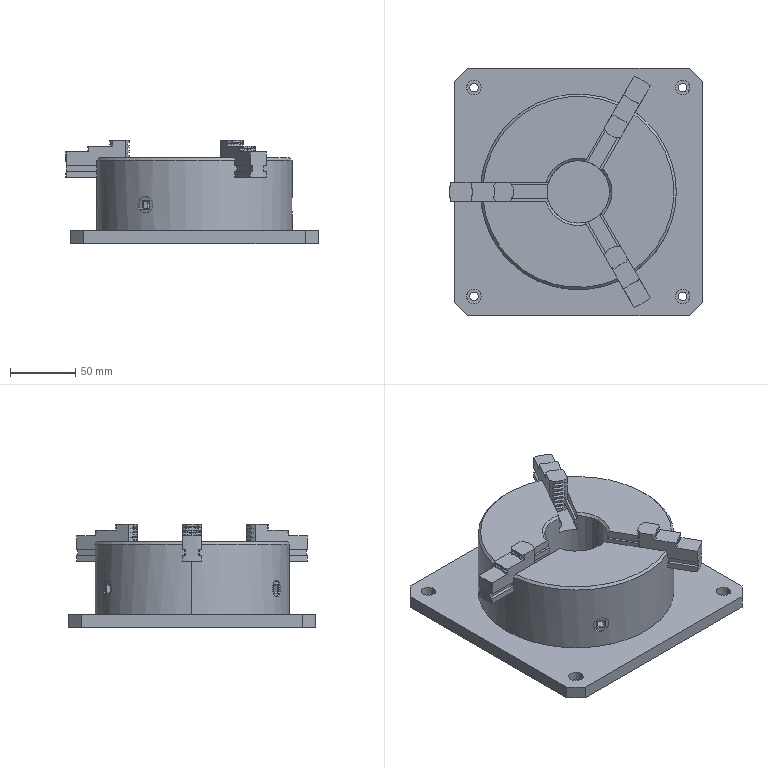Part | SolidWorks | features BaseBody 4, MoveCopyBody 3, Chamfer 1, HoleWzd 1, ICE 1, MoveFace 1, Scale 1 | 4 solids | 320 faces | box 193.6 x 190 x 79.5 mm | volume 1119464 mm3 | plane 214 | cylinder 73 | cone 33 | commonest cylinder face diameters 33.6 x18 51.6 x12 6.6 x8 11 x8 5.1 x6 6 x6